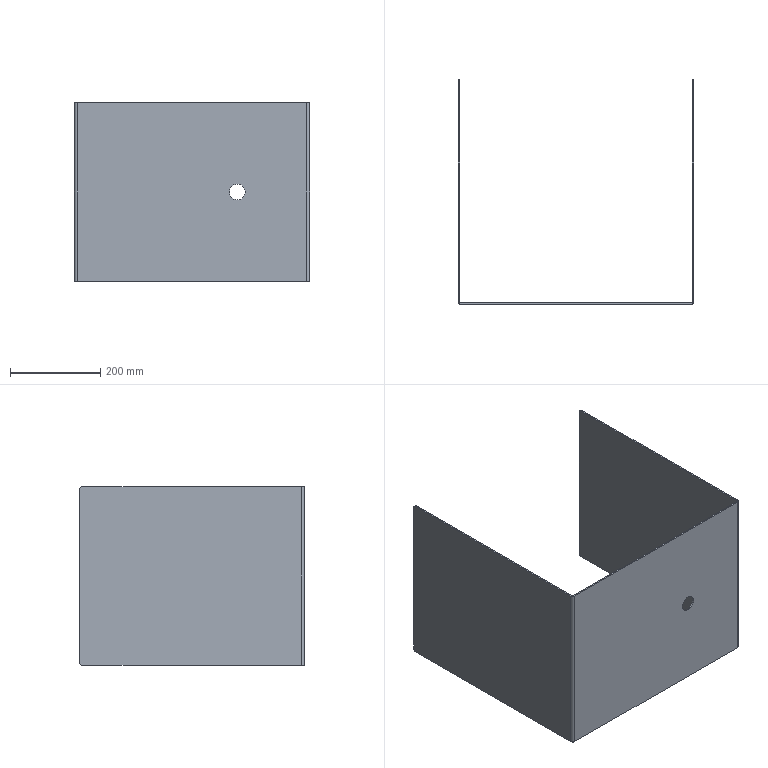Part | SolidWorks | features ICE 2, FlatPattern 1, SMBaseFlange 1, SheetMetal 1 | 1 solid | 28 faces | box 520 x 497 x 394 mm | volume 1774939 mm3 | plane 18 | cylinder 10 | commonest cylinder face diameters 10 x4 6 x2 12 x2 35 x2
STEP:
#1=CARTESIAN_POINT('',(360.,3.,179.5));
#2=VERTEX_POINT('',#1);
#3=CARTESIAN_POINT('',(360.,3.,214.5));
#4=VERTEX_POINT('',#3);
#5=CARTESIAN_POINT('',(360.,3.,197.));
#6=DIRECTION('',(0.,1.,0.));
#7=DIRECTION('',(0.,0.,1.));
#8=AXIS2_PLACEMENT_3D('',#5,#6,#7);
#9=CIRCLE('',#8,17.5);
#10=EDGE_CURVE('',#2,#4,#9,.T.);
#11=ORIENTED_EDGE('',*,*,#10,.T.);
#12=CARTESIAN_POINT('',(360.,0.,214.5));
#13=VERTEX_POINT('',#12);
#14=CARTESIAN_POINT('',(360.,10.,214.5));
#15=DIRECTION('',(0.,-1.,0.));
#16=VECTOR('',#15,1000.);
#17=LINE('',#14,#16);
#18=EDGE_CURVE('',#4,#13,#17,.T.);
#19=ORIENTED_EDGE('',*,*,#18,.T.);
#20=CARTESIAN_POINT('',(360.,0.,179.5));
#21=VERTEX_POINT('',#20);
#22=CARTESIAN_POINT('',(360.,0.,197.));
#23=DIRECTION('',(0.,-1.,0.));
#24=DIRECTION('',(0.,0.,-1.));
#25=AXIS2_PLACEMENT_3D('',#22,#23,#24);
#26=CIRCLE('',#25,17.5);
#27=EDGE_CURVE('',#13,#21,#26,.T.);
#28=ORIENTED_EDGE('',*,*,#27,.T.);
#29=CARTESIAN_POINT('',(360.,10.,179.5));
#30=DIRECTION('',(0.,-1.,0.));
#31=VECTOR('',#30,1000.);
#32=LINE('',#29,#31);
#33=EDGE_CURVE('',#2,#21,#32,.T.);
#34=ORIENTED_EDGE('',*,*,#33,.F.);
#35=EDGE_LOOP('',(#11,#19,#28,#34));
#36=FACE_OUTER_BOUND('',#35,.T.);
#37=CARTESIAN_POINT('',(360.,10.,197.));
#38=DIRECTION('',(0.,-1.,0.));
#39=DIRECTION('',(0.,0.,-1.));
#40=AXIS2_PLACEMENT_3D('',#37,#38,#39);
#41=CYLINDRICAL_SURFACE('',#40,17.5);
#42=ADVANCED_FACE('',(#36),#41,.F.);
#43=CARTESIAN_POINT('',(520.,492.,0.));
#44=VERTEX_POINT('',#43);
#45=CARTESIAN_POINT('',(520.,497.,5.));
#46=VERTEX_POINT('',#45);
#47=CARTESIAN_POINT('',(520.,492.,5.));
#48=DIRECTION('',(1.,0.,0.));
#49=DIRECTION('',(0.,0.,1.));
#50=AXIS2_PLACEMENT_3D('',#47,#48,#49);
#51=CIRCLE('',#50,5.);
#52=EDGE_CURVE('',#44,#46,#51,.T.);
#53=ORIENTED_EDGE('',*,*,#52,.T.);
#54=CARTESIAN_POINT('',(520.,497.,389.));
#55=VERTEX_POINT('',#54);
#56=CARTESIAN_POINT('',(520.,497.,394.));
#57=DIRECTION('',(0.,0.,-1.));
#58=VECTOR('',#57,1000.);
#59=LINE('',#56,#58);
#60=EDGE_CURVE('',#55,#46,#59,.T.);
#61=ORIENTED_EDGE('',*,*,#60,.F.);
#62=CARTESIAN_POINT('',(520.,492.,394.));
#63=VERTEX_POINT('',#62);
#64=CARTESIAN_POINT('',(520.,492.,389.));
#65=DIRECTION('',(1.,0.,0.));
#66=DIRECTION('',(0.,0.,1.));
#67=AXIS2_PLACEMENT_3D('',#64,#65,#66);
#68=CIRCLE('',#67,5.);
#69=EDGE_CURVE('',#55,#63,#68,.T.);
#70=ORIENTED_EDGE('',*,*,#69,.T.);
#71=CARTESIAN_POINT('',(520.,6.,394.));
#72=VERTEX_POINT('',#71);
#73=CARTESIAN_POINT('',(520.,0.,394.));
#74=DIRECTION('',(0.,1.,0.));
#75=VECTOR('',#74,1000.);
#76=LINE('',#73,#75);
#77=EDGE_CURVE('',#72,#63,#76,.T.);
#78=ORIENTED_EDGE('',*,*,#77,.F.);
#79=CARTESIAN_POINT('',(520.,6.,0.));
#80=VERTEX_POINT('',#79);
#81=CARTESIAN_POINT('',(520.,6.,394.));
#82=DIRECTION('',(0.,0.,-1.));
#83=VECTOR('',#82,1000.);
#84=LINE('',#81,#83);
#85=EDGE_CURVE('',#72,#80,#84,.T.);
#86=ORIENTED_EDGE('',*,*,#85,.T.);
#87=CARTESIAN_POINT('',(520.,0.,0.));
#88=DIRECTION('',(0.,1.,0.));
#89=VECTOR('',#88,1000.);
#90=LINE('',#87,#89);
#91=EDGE_CURVE('',#80,#44,#90,.T.);
#92=ORIENTED_EDGE('',*,*,#91,.T.);
#93=EDGE_LOOP('',(#53,#61,#70,#78,#86,#92));
#94=FACE_OUTER_BOUND('',#93,.T.);
#95=CARTESIAN_POINT('',(520.,0.,394.));
#96=DIRECTION('',(-1.,0.,0.));
#97=DIRECTION('',(0.,0.,1.));
#98=AXIS2_PLACEMENT_3D('',#95,#96,#97);
#99=PLANE('',#98);
#100=ADVANCED_FACE('',(#94),#99,.F.);
#101=CARTESIAN_POINT('',(517.,497.,389.));
#102=VERTEX_POINT('',#101);
#103=CARTESIAN_POINT('',(517.,497.,5.));
#104=VERTEX_POINT('',#103);
#105=CARTESIAN_POINT('',(517.,497.,394.));
#106=DIRECTION('',(0.,0.,-1.));
#107=VECTOR('',#106,1000.);
#108=LINE('',#105,#107);
#109=EDGE_CURVE('',#102,#104,#108,.T.);
#110=ORIENTED_EDGE('',*,*,#109,.T.);
#111=CARTESIAN_POINT('',(517.,492.,0.));
#112=VERTEX_POINT('',#111);
#113=CARTESIAN_POINT('',(517.,492.,5.));
#114=DIRECTION('',(1.,0.,0.));
#115=DIRECTION('',(0.,0.,1.));
#116=AXIS2_PLACEMENT_3D('',#113,#114,#115);
#117=CIRCLE('',#116,5.);
#118=EDGE_CURVE('',#112,#104,#117,.T.);
#119=ORIENTED_EDGE('',*,*,#118,.F.);
#120=CARTESIAN_POINT('',(517.,6.,0.));
#121=VERTEX_POINT('',#120);
#122=CARTESIAN_POINT('',(517.,0.,0.));
#123=DIRECTION('',(0.,1.,0.));
#124=VECTOR('',#123,1000.);
#125=LINE('',#122,#124);
#126=EDGE_CURVE('',#121,#112,#125,.T.);
#127=ORIENTED_EDGE('',*,*,#126,.F.);
#128=CARTESIAN_POINT('',(517.,6.,394.));
#129=VERTEX_POINT('',#128);
#130=CARTESIAN_POINT('',(517.,6.,394.));
#131=DIRECTION('',(0.,0.,-1.));
#132=VECTOR('',#131,1000.);
#133=LINE('',#130,#132);
#134=EDGE_CURVE('',#129,#121,#133,.T.);
#135=ORIENTED_EDGE('',*,*,#134,.F.);
#136=CARTESIAN_POINT('',(517.,492.,394.));
#137=VERTEX_POINT('',#136);
#138=CARTESIAN_POINT('',(517.,0.,394.));
#139=DIRECTION('',(0.,1.,0.));
#140=VECTOR('',#139,1000.);
#141=LINE('',#138,#140);
#142=EDGE_CURVE('',#129,#137,#141,.T.);
#143=ORIENTED_EDGE('',*,*,#142,.T.);
#144=CARTESIAN_POINT('',(517.,492.,389.));
#145=DIRECTION('',(1.,0.,0.));
#146=DIRECTION('',(0.,0.,1.));
#147=AXIS2_PLACEMENT_3D('',#144,#145,#146);
#148=CIRCLE('',#147,5.);
#149=EDGE_CURVE('',#102,#137,#148,.T.);
#150=ORIENTED_EDGE('',*,*,#149,.F.);
#151=EDGE_LOOP('',(#110,#119,#127,#135,#143,#150));
#152=FACE_OUTER_BOUND('',#151,.T.);
#153=CARTESIAN_POINT('',(517.,0.,394.));
#154=DIRECTION('',(-1.,0.,0.));
#155=DIRECTION('',(0.,0.,1.));
#156=AXIS2_PLACEMENT_3D('',#153,#154,#155);
#157=PLANE('',#156);
#158=ADVANCED_FACE('',(#152),#157,.T.);
#159=ORIENTED_EDGE('',*,*,#60,.T.);
#160=CARTESIAN_POINT('',(517.,497.,5.));
#161=DIRECTION('',(1.,0.,0.));
#162=VECTOR('',#161,1000.);
#163=LINE('',#160,#162);
#164=EDGE_CURVE('',#104,#46,#163,.T.);
#165=ORIENTED_EDGE('',*,*,#164,.F.);
#166=ORIENTED_EDGE('',*,*,#109,.F.);
#167=CARTESIAN_POINT('',(517.,497.,389.));
#168=DIRECTION('',(1.,0.,0.));
#169=VECTOR('',#168,1000.);
#170=LINE('',#167,#169);
#171=EDGE_CURVE('',#102,#55,#170,.T.);
#172=ORIENTED_EDGE('',*,*,#171,.T.);
#173=EDGE_LOOP('',(#159,#165,#166,#172));
#174=FACE_OUTER_BOUND('',#173,.T.);
#175=CARTESIAN_POINT('',(517.,497.,394.));
#176=DIRECTION('',(0.,1.,0.));
#177=DIRECTION('',(0.,0.,1.));
#178=AXIS2_PLACEMENT_3D('',#175,#176,#177);
#179=PLANE('',#178);
#180=ADVANCED_FACE('',(#174),#179,.T.);
#181=CARTESIAN_POINT('',(3.,492.,0.));
#182=VERTEX_POINT('',#181);
#183=CARTESIAN_POINT('',(3.,6.,0.));
#184=VERTEX_POINT('',#183);
#185=CARTESIAN_POINT('',(3.,0.,0.));
#186=DIRECTION('',(0.,-1.,0.));
#187=VECTOR('',#186,1000.);
#188=LINE('',#185,#187);
#189=EDGE_CURVE('',#182,#184,#188,.T.);
#190=ORIENTED_EDGE('',*,*,#189,.F.);
#191=CARTESIAN_POINT('',(3.,497.,5.));
#192=VERTEX_POINT('',#191);
#193=CARTESIAN_POINT('',(3.,492.,5.));
#194=DIRECTION('',(-1.,0.,0.));
#195=DIRECTION('',(0.,0.,-1.));
#196=AXIS2_PLACEMENT_3D('',#193,#194,#195);
#197=CIRCLE('',#196,5.);
#198=EDGE_CURVE('',#192,#182,#197,.T.);
#199=ORIENTED_EDGE('',*,*,#198,.F.);
#200=CARTESIAN_POINT('',(3.,497.,389.));
#201=VERTEX_POINT('',#200);
#202=CARTESIAN_POINT('',(3.,497.,394.));
#203=DIRECTION('',(0.,0.,-1.));
#204=VECTOR('',#203,1000.);
#205=LINE('',#202,#204);
#206=EDGE_CURVE('',#201,#192,#205,.T.);
#207=ORIENTED_EDGE('',*,*,#206,.F.);
#208=CARTESIAN_POINT('',(3.,492.,394.));
#209=VERTEX_POINT('',#208);
#210=CARTESIAN_POINT('',(3.,492.,389.));
#211=DIRECTION('',(-1.,0.,0.));
#212=DIRECTION('',(0.,0.,-1.));
#213=AXIS2_PLACEMENT_3D('',#210,#211,#212);
#214=CIRCLE('',#213,5.);
#215=EDGE_CURVE('',#209,#201,#214,.T.);
#216=ORIENTED_EDGE('',*,*,#215,.F.);
#217=CARTESIAN_POINT('',(3.,6.,394.));
#218=VERTEX_POINT('',#217);
#219=CARTESIAN_POINT('',(3.,0.,394.));
#220=DIRECTION('',(0.,-1.,0.));
#221=VECTOR('',#220,1000.);
#222=LINE('',#219,#221);
#223=EDGE_CURVE('',#209,#218,#222,.T.);
#224=ORIENTED_EDGE('',*,*,#223,.T.);
#225=CARTESIAN_POINT('',(3.,6.,394.));
#226=DIRECTION('',(0.,0.,-1.));
#227=VECTOR('',#226,1000.);
#228=LINE('',#225,#227);
#229=EDGE_CURVE('',#218,#184,#228,.T.);
#230=ORIENTED_EDGE('',*,*,#229,.T.);
#231=EDGE_LOOP('',(#190,#199,#207,#216,#224,#230));
#232=FACE_OUTER_BOUND('',#231,.T.);
#233=CARTESIAN_POINT('',(3.,0.,394.));
#234=DIRECTION('',(1.,0.,0.));
#235=DIRECTION('',(0.,0.,-1.));
#236=AXIS2_PLACEMENT_3D('',#233,#234,#235);
#237=PLANE('',#236);
#238=ADVANCED_FACE('',(#232),#237,.T.);
#239=CARTESIAN_POINT('',(0.,497.,5.));
#240=VERTEX_POINT('',#239);
#241=CARTESIAN_POINT('',(0.,492.,0.));
#242=VERTEX_POINT('',#241);
#243=CARTESIAN_POINT('',(0.,492.,5.));
#244=DIRECTION('',(-1.,0.,0.));
#245=DIRECTION('',(0.,0.,-1.));
#246=AXIS2_PLACEMENT_3D('',#243,#244,#245);
#247=CIRCLE('',#246,5.);
#248=EDGE_CURVE('',#240,#242,#247,.T.);
#249=ORIENTED_EDGE('',*,*,#248,.T.);
#250=CARTESIAN_POINT('',(0.,6.,0.));
#251=VERTEX_POINT('',#250);
#252=CARTESIAN_POINT('',(0.,0.,0.));
#253=DIRECTION('',(0.,-1.,0.));
#254=VECTOR('',#253,1000.);
#255=LINE('',#252,#254);
#256=EDGE_CURVE('',#242,#251,#255,.T.);
#257=ORIENTED_EDGE('',*,*,#256,.T.);
#258=CARTESIAN_POINT('',(0.,6.,394.));
#259=VERTEX_POINT('',#258);
#260=CARTESIAN_POINT('',(0.,6.,394.));
#261=DIRECTION('',(0.,0.,-1.));
#262=VECTOR('',#261,1000.);
#263=LINE('',#260,#262);
#264=EDGE_CURVE('',#259,#251,#263,.T.);
#265=ORIENTED_EDGE('',*,*,#264,.F.);
#266=CARTESIAN_POINT('',(0.,492.,394.));
#267=VERTEX_POINT('',#266);
#268=CARTESIAN_POINT('',(0.,0.,394.));
#269=DIRECTION('',(0.,-1.,0.));
#270=VECTOR('',#269,1000.);
#271=LINE('',#268,#270);
#272=EDGE_CURVE('',#267,#259,#271,.T.);
#273=ORIENTED_EDGE('',*,*,#272,.F.);
#274=CARTESIAN_POINT('',(0.,497.,389.));
#275=VERTEX_POINT('',#274);
#276=CARTESIAN_POINT('',(0.,492.,389.));
#277=DIRECTION('',(-1.,0.,0.));
#278=DIRECTION('',(0.,0.,-1.));
#279=AXIS2_PLACEMENT_3D('',#276,#277,#278);
#280=CIRCLE('',#279,5.);
#281=EDGE_CURVE('',#267,#275,#280,.T.);
#282=ORIENTED_EDGE('',*,*,#281,.T.);
#283=CARTESIAN_POINT('',(0.,497.,394.));
#284=DIRECTION('',(0.,0.,-1.));
#285=VECTOR('',#284,1000.);
#286=LINE('',#283,#285);
#287=EDGE_CURVE('',#275,#240,#286,.T.);
#288=ORIENTED_EDGE('',*,*,#287,.T.);
#289=EDGE_LOOP('',(#249,#257,#265,#273,#282,#288));
#290=FACE_OUTER_BOUND('',#289,.T.);
#291=CARTESIAN_POINT('',(0.,0.,394.));
#292=DIRECTION('',(1.,0.,0.));
#293=DIRECTION('',(0.,0.,-1.));
#294=AXIS2_PLACEMENT_3D('',#291,#292,#293);
#295=PLANE('',#294);
#296=ADVANCED_FACE('',(#290),#295,.F.);
#297=ORIENTED_EDGE('',*,*,#77,.T.);
#298=CARTESIAN_POINT('',(517.,492.,394.));
#299=DIRECTION('',(1.,0.,0.));
#300=VECTOR('',#299,1000.);
#301=LINE('',#298,#300);
#302=EDGE_CURVE('',#137,#63,#301,.T.);
#303=ORIENTED_EDGE('',*,*,#302,.F.);
#304=ORIENTED_EDGE('',*,*,#142,.F.);
#305=CARTESIAN_POINT('',(517.,6.,394.));
#306=DIRECTION('',(1.,0.,0.));
#307=VECTOR('',#306,1000.);
#308=LINE('',#305,#307);
#309=EDGE_CURVE('',#129,#72,#308,.T.);
#310=ORIENTED_EDGE('',*,*,#309,.T.);
#311=EDGE_LOOP('',(#297,#303,#304,#310));
#312=FACE_OUTER_BOUND('',#311,.T.);
#313=CARTESIAN_POINT('',(514.,6.,394.));
#314=DIRECTION('',(0.,0.,1.));
#315=DIRECTION('',(1.,0.,0.));
#316=AXIS2_PLACEMENT_3D('',#313,#314,#315);
#317=PLANE('',#316);
#318=ADVANCED_FACE('',(#312),#317,.T.);
#319=CARTESIAN_POINT('',(3.,497.,5.));
#320=DIRECTION('',(-1.,0.,0.));
#321=VECTOR('',#320,1000.);
#322=LINE('',#319,#321);
#323=EDGE_CURVE('',#192,#240,#322,.T.);
#324=ORIENTED_EDGE('',*,*,#323,.T.);
#325=ORIENTED_EDGE('',*,*,#287,.F.);
#326=CARTESIAN_POINT('',(3.,497.,389.));
#327=DIRECTION('',(-1.,0.,0.));
#328=VECTOR('',#327,1000.);
#329=LINE('',#326,#328);
#330=EDGE_CURVE('',#201,#275,#329,.T.);
#331=ORIENTED_EDGE('',*,*,#330,.F.);
#332=ORIENTED_EDGE('',*,*,#206,.T.);
#333=EDGE_LOOP('',(#324,#325,#331,#332));
#334=FACE_OUTER_BOUND('',#333,.T.);
#335=CARTESIAN_POINT('',(0.,497.,394.));
#336=DIRECTION('',(0.,1.,0.));
#337=DIRECTION('',(0.,0.,1.));
#338=AXIS2_PLACEMENT_3D('',#335,#336,#337);
#339=PLANE('',#338);
#340=ADVANCED_FACE('',(#334),#339,.T.);
#341=CARTESIAN_POINT('',(0.,6.,394.));
#342=DIRECTION('',(1.,0.,0.));
#343=VECTOR('',#342,1000.);
#344=LINE('',#341,#343);
#345=EDGE_CURVE('',#259,#218,#344,.T.);
#346=ORIENTED_EDGE('',*,*,#345,.F.);
#347=CARTESIAN_POINT('',(6.,0.,394.));
#348=VERTEX_POINT('',#347);
#349=CARTESIAN_POINT('',(6.,6.,394.));
#350=DIRECTION('',(0.,0.,1.));
#351=DIRECTION('',(-1.,0.,0.));
#352=AXIS2_PLACEMENT_3D('',#349,#350,#351);
#353=CIRCLE('',#352,6.);
#354=EDGE_CURVE('',#259,#348,#353,.T.);
#355=ORIENTED_EDGE('',*,*,#354,.T.);
#356=CARTESIAN_POINT('',(6.,3.,394.));
#357=VERTEX_POINT('',#356);
#358=CARTESIAN_POINT('',(6.,3.,394.));
#359=DIRECTION('',(0.,-1.,0.));
#360=VECTOR('',#359,1000.);
#361=LINE('',#358,#360);
#362=EDGE_CURVE('',#357,#348,#361,.T.);
#363=ORIENTED_EDGE('',*,*,#362,.F.);
#364=CARTESIAN_POINT('',(6.,6.,394.));
#365=DIRECTION('',(0.,0.,1.));
#366=DIRECTION('',(1.,0.,0.));
#367=AXIS2_PLACEMENT_3D('',#364,#365,#366);
#368=CIRCLE('',#367,3.);
#369=EDGE_CURVE('',#218,#357,#368,.T.);
#370=ORIENTED_EDGE('',*,*,#369,.F.);
#371=EDGE_LOOP('',(#346,#355,#363,#370));
#372=FACE_OUTER_BOUND('',#371,.T.);
#373=CARTESIAN_POINT('',(0.,6.,394.));
#374=DIRECTION('',(0.,0.,1.));
#375=DIRECTION('',(1.,0.,0.));
#376=AXIS2_PLACEMENT_3D('',#373,#374,#375);
#377=PLANE('',#376);
#378=ADVANCED_FACE('',(#372),#377,.T.);
#379=CARTESIAN_POINT('',(3.,492.,394.));
#380=DIRECTION('',(-1.,0.,0.));
#381=VECTOR('',#380,1000.);
#382=LINE('',#379,#381);
#383=EDGE_CURVE('',#209,#267,#382,.T.);
#384=ORIENTED_EDGE('',*,*,#383,.T.);
#385=ORIENTED_EDGE('',*,*,#272,.T.);
#386=ORIENTED_EDGE('',*,*,#345,.T.);
#387=ORIENTED_EDGE('',*,*,#223,.F.);
#388=EDGE_LOOP('',(#384,#385,#386,#387));
#389=FACE_OUTER_BOUND('',#388,.T.);
#390=CARTESIAN_POINT('',(6.,3.,394.));
#391=DIRECTION('',(0.,0.,1.));
#392=DIRECTION('',(1.,0.,0.));
#393=AXIS2_PLACEMENT_3D('',#390,#391,#392);
#394=PLANE('',#393);
#395=ADVANCED_FACE('',(#389),#394,.T.);
#396=CARTESIAN_POINT('',(6.,0.,0.));
#397=VERTEX_POINT('',#396);
#398=CARTESIAN_POINT('',(6.,3.,0.));
#399=VERTEX_POINT('',#398);
#400=CARTESIAN_POINT('',(6.,0.,0.));
#401=DIRECTION('',(0.,1.,0.));
#402=VECTOR('',#401,1000.);
#403=LINE('',#400,#402);
#404=EDGE_CURVE('',#397,#399,#403,.T.);
#405=ORIENTED_EDGE('',*,*,#404,.F.);
#406=CARTESIAN_POINT('',(6.,6.,0.));
#407=DIRECTION('',(0.,0.,1.));
#408=DIRECTION('',(-1.,0.,0.));
#409=AXIS2_PLACEMENT_3D('',#406,#407,#408);
#410=CIRCLE('',#409,6.);
#411=EDGE_CURVE('',#251,#397,#410,.T.);
#412=ORIENTED_EDGE('',*,*,#411,.F.);
#413=CARTESIAN_POINT('',(3.,6.,0.));
#414=DIRECTION('',(-1.,0.,0.));
#415=VECTOR('',#414,1000.);
#416=LINE('',#413,#415);
#417=EDGE_CURVE('',#184,#251,#416,.T.);
#418=ORIENTED_EDGE('',*,*,#417,.F.);
#419=CARTESIAN_POINT('',(6.,6.,0.));
#420=DIRECTION('',(0.,0.,1.));
#421=DIRECTION('',(1.,0.,0.));
#422=AXIS2_PLACEMENT_3D('',#419,#420,#421);
#423=CIRCLE('',#422,3.);
#424=EDGE_CURVE('',#184,#399,#423,.T.);
#425=ORIENTED_EDGE('',*,*,#424,.T.);
#426=EDGE_LOOP('',(#405,#412,#418,#425));
#427=FACE_OUTER_BOUND('',#426,.T.);
#428=CARTESIAN_POINT('',(6.,0.,0.));
#429=DIRECTION('',(0.,0.,-1.));
#430=DIRECTION('',(-1.,0.,0.));
#431=AXIS2_PLACEMENT_3D('',#428,#429,#430);
#432=PLANE('',#431);
#433=ADVANCED_FACE('',(#427),#432,.T.);
#434=CARTESIAN_POINT('',(514.,0.,0.));
#435=VERTEX_POINT('',#434);
#436=CARTESIAN_POINT('',(0.,0.,0.));
#437=DIRECTION('',(1.,0.,0.));
#438=VECTOR('',#437,1000.);
#439=LINE('',#436,#438);
#440=EDGE_CURVE('',#397,#435,#439,.T.);
#441=ORIENTED_EDGE('',*,*,#440,.F.);
#442=ORIENTED_EDGE('',*,*,#404,.T.);
#443=CARTESIAN_POINT('',(514.,3.,0.));
#444=VERTEX_POINT('',#443);
#445=CARTESIAN_POINT('',(0.,3.,0.));
#446=DIRECTION('',(1.,0.,0.));
#447=VECTOR('',#446,1000.);
#448=LINE('',#445,#447);
#449=EDGE_CURVE('',#399,#444,#448,.T.);
#450=ORIENTED_EDGE('',*,*,#449,.T.);
#451=CARTESIAN_POINT('',(514.,3.,0.));
#452=DIRECTION('',(0.,-1.,0.));
#453=VECTOR('',#452,1000.);
#454=LINE('',#451,#453);
#455=EDGE_CURVE('',#444,#435,#454,.T.);
#456=ORIENTED_EDGE('',*,*,#455,.T.);
#457=EDGE_LOOP('',(#441,#442,#450,#456));
#458=FACE_OUTER_BOUND('',#457,.T.);
#459=CARTESIAN_POINT('',(3.,6.,0.));
#460=DIRECTION('',(0.,0.,-1.));
#461=DIRECTION('',(-1.,0.,0.));
#462=AXIS2_PLACEMENT_3D('',#459,#460,#461);
#463=PLANE('',#462);
#464=ADVANCED_FACE('',(#458),#463,.T.);
#465=CARTESIAN_POINT('',(514.,0.,394.));
#466=VERTEX_POINT('',#465);
#467=CARTESIAN_POINT('',(514.,3.,394.));
#468=VERTEX_POINT('',#467);
#469=CARTESIAN_POINT('',(514.,0.,394.));
#470=DIRECTION('',(0.,1.,0.));
#471=VECTOR('',#470,1000.);
#472=LINE('',#469,#471);
#473=EDGE_CURVE('',#466,#468,#472,.T.);
#474=ORIENTED_EDGE('',*,*,#473,.F.);
#475=CARTESIAN_POINT('',(514.,6.,394.));
#476=DIRECTION('',(0.,0.,1.));
#477=DIRECTION('',(-1.,0.,0.));
#478=AXIS2_PLACEMENT_3D('',#475,#476,#477);
#479=CIRCLE('',#478,6.);
#480=EDGE_CURVE('',#466,#72,#479,.T.);
#481=ORIENTED_EDGE('',*,*,#480,.T.);
#482=ORIENTED_EDGE('',*,*,#309,.F.);
#483=CARTESIAN_POINT('',(514.,6.,394.));
#484=DIRECTION('',(0.,0.,1.));
#485=DIRECTION('',(1.,0.,0.));
#486=AXIS2_PLACEMENT_3D('',#483,#484,#485);
#487=CIRCLE('',#486,3.);
#488=EDGE_CURVE('',#468,#129,#487,.T.);
#489=ORIENTED_EDGE('',*,*,#488,.F.);
#490=EDGE_LOOP('',(#474,#481,#482,#489));
#491=FACE_OUTER_BOUND('',#490,.T.);
#492=CARTESIAN_POINT('',(514.,0.,394.));
#493=DIRECTION('',(0.,0.,1.));
#494=DIRECTION('',(1.,0.,0.));
#495=AXIS2_PLACEMENT_3D('',#492,#493,#494);
#496=PLANE('',#495);
#497=ADVANCED_FACE('',(#491),#496,.T.);
#498=CARTESIAN_POINT('',(0.,0.,394.));
#499=DIRECTION('',(1.,0.,0.));
#500=VECTOR('',#499,1000.);
#501=LINE('',#498,#500);
#502=EDGE_CURVE('',#348,#466,#501,.T.);
#503=ORIENTED_EDGE('',*,*,#502,.T.);
#504=ORIENTED_EDGE('',*,*,#473,.T.);
#505=CARTESIAN_POINT('',(0.,3.,394.));
#506=DIRECTION('',(1.,0.,0.));
#507=VECTOR('',#506,1000.);
#508=LINE('',#505,#507);
#509=EDGE_CURVE('',#357,#468,#508,.T.);
#510=ORIENTED_EDGE('',*,*,#509,.F.);
#511=ORIENTED_EDGE('',*,*,#362,.T.);
#512=EDGE_LOOP('',(#503,#504,#510,#511));
#513=FACE_OUTER_BOUND('',#512,.T.);
#514=CARTESIAN_POINT('',(517.,6.,394.));
#515=DIRECTION('',(0.,0.,1.));
#516=DIRECTION('',(1.,0.,0.));
#517=AXIS2_PLACEMENT_3D('',#514,#515,#516);
#518=PLANE('',#517);
#519=ADVANCED_FACE('',(#513),#518,.T.);
#520=CARTESIAN_POINT('',(520.,6.,0.));
#521=DIRECTION('',(-1.,0.,0.));
#522=VECTOR('',#521,1000.);
#523=LINE('',#520,#522);
#524=EDGE_CURVE('',#80,#121,#523,.T.);
#525=ORIENTED_EDGE('',*,*,#524,.F.);
#526=CARTESIAN_POINT('',(514.,6.,0.));
#527=DIRECTION('',(0.,0.,1.));
#528=DIRECTION('',(-1.,0.,0.));
#529=AXIS2_PLACEMENT_3D('',#526,#527,#528);
#530=CIRCLE('',#529,6.);
#531=EDGE_CURVE('',#435,#80,#530,.T.);
#532=ORIENTED_EDGE('',*,*,#531,.F.);
#533=ORIENTED_EDGE('',*,*,#455,.F.);
#534=CARTESIAN_POINT('',(514.,6.,0.));
#535=DIRECTION('',(0.,0.,1.));
#536=DIRECTION('',(1.,0.,0.));
#537=AXIS2_PLACEMENT_3D('',#534,#535,#536);
#538=CIRCLE('',#537,3.);
#539=EDGE_CURVE('',#444,#121,#538,.T.);
#540=ORIENTED_EDGE('',*,*,#539,.T.);
#541=EDGE_LOOP('',(#525,#532,#533,#540));
#542=FACE_OUTER_BOUND('',#541,.T.);
#543=CARTESIAN_POINT('',(520.,6.,0.));
#544=DIRECTION('',(0.,0.,-1.));
#545=DIRECTION('',(-1.,0.,0.));
#546=AXIS2_PLACEMENT_3D('',#543,#544,#545);
#547=PLANE('',#546);
#548=ADVANCED_FACE('',(#542),#547,.T.);
#549=CARTESIAN_POINT('',(517.,492.,0.));
#550=DIRECTION('',(1.,0.,0.));
#551=VECTOR('',#550,1000.);
#552=LINE('',#549,#551);
#553=EDGE_CURVE('',#112,#44,#552,.T.);
#554=ORIENTED_EDGE('',*,*,#553,.T.);
#555=ORIENTED_EDGE('',*,*,#91,.F.);
#556=ORIENTED_EDGE('',*,*,#524,.T.);
#557=ORIENTED_EDGE('',*,*,#126,.T.);
#558=EDGE_LOOP('',(#554,#555,#556,#557));
#559=FACE_OUTER_BOUND('',#558,.T.);
#560=CARTESIAN_POINT('',(514.,3.,0.));
#561=DIRECTION('',(0.,0.,-1.));
#562=DIRECTION('',(-1.,0.,0.));
#563=AXIS2_PLACEMENT_3D('',#560,#561,#562);
#564=PLANE('',#563);
#565=ADVANCED_FACE('',(#559),#564,.T.);
#566=ORIENTED_EDGE('',*,*,#539,.F.);
#567=CARTESIAN_POINT('',(514.,3.,394.));
#568=DIRECTION('',(0.,0.,-1.));
#569=VECTOR('',#568,1000.);
#570=LINE('',#567,#569);
#571=EDGE_CURVE('',#468,#444,#570,.T.);
#572=ORIENTED_EDGE('',*,*,#571,.F.);
#573=ORIENTED_EDGE('',*,*,#488,.T.);
#574=ORIENTED_EDGE('',*,*,#134,.T.);
#575=EDGE_LOOP('',(#566,#572,#573,#574));
#576=FACE_OUTER_BOUND('',#575,.T.);
#577=CARTESIAN_POINT('',(514.,6.,394.));
#578=DIRECTION('',(0.,0.,-1.));
#579=DIRECTION('',(-1.,0.,0.));
#580=AXIS2_PLACEMENT_3D('',#577,#578,#579);
#581=CYLINDRICAL_SURFACE('',#580,3.);
#582=ADVANCED_FACE('',(#576),#581,.F.);
#583=ORIENTED_EDGE('',*,*,#10,.F.);
#584=CARTESIAN_POINT('',(360.,3.,197.));
#585=DIRECTION('',(0.,1.,0.));
#586=DIRECTION('',(0.,0.,1.));
#587=AXIS2_PLACEMENT_3D('',#584,#585,#586);
#588=CIRCLE('',#587,17.5);
#589=EDGE_CURVE('',#4,#2,#588,.T.);
#590=ORIENTED_EDGE('',*,*,#589,.F.);
#591=EDGE_LOOP('',(#583,#590));
#592=FACE_BOUND('',#591,.T.);
#593=ORIENTED_EDGE('',*,*,#449,.F.);
#594=CARTESIAN_POINT('',(6.,3.,394.));
#595=DIRECTION('',(0.,0.,-1.));
#596=VECTOR('',#595,1000.);
#597=LINE('',#594,#596);
#598=EDGE_CURVE('',#357,#399,#597,.T.);
#599=ORIENTED_EDGE('',*,*,#598,.F.);
#600=ORIENTED_EDGE('',*,*,#509,.T.);
#601=ORIENTED_EDGE('',*,*,#571,.T.);
#602=EDGE_LOOP('',(#593,#599,#600,#601));
#603=FACE_OUTER_BOUND('',#602,.T.);
#604=CARTESIAN_POINT('',(0.,3.,394.));
#605=DIRECTION('',(0.,1.,0.));
#606=DIRECTION('',(0.,0.,1.));
#607=AXIS2_PLACEMENT_3D('',#604,#605,#606);
#608=PLANE('',#607);
#609=ADVANCED_FACE('',(#592,#603),#608,.T.);
#610=ORIENTED_EDGE('',*,*,#424,.F.);
#611=ORIENTED_EDGE('',*,*,#229,.F.);
#612=ORIENTED_EDGE('',*,*,#369,.T.);
#613=ORIENTED_EDGE('',*,*,#598,.T.);
#614=EDGE_LOOP('',(#610,#611,#612,#613));
#615=FACE_OUTER_BOUND('',#614,.T.);
#616=CARTESIAN_POINT('',(6.,6.,394.));
#617=DIRECTION('',(0.,0.,-1.));
#618=DIRECTION('',(-1.,0.,0.));
#619=AXIS2_PLACEMENT_3D('',#616,#617,#618);
#620=CYLINDRICAL_SURFACE('',#619,3.);
#621=ADVANCED_FACE('',(#615),#620,.F.);
#622=ORIENTED_EDGE('',*,*,#411,.T.);
#623=CARTESIAN_POINT('',(6.,0.,394.));
#624=DIRECTION('',(0.,0.,-1.));
#625=VECTOR('',#624,1000.);
#626=LINE('',#623,#625);
#627=EDGE_CURVE('',#348,#397,#626,.T.);
#628=ORIENTED_EDGE('',*,*,#627,.F.);
#629=ORIENTED_EDGE('',*,*,#354,.F.);
#630=ORIENTED_EDGE('',*,*,#264,.T.);
#631=EDGE_LOOP('',(#622,#628,#629,#630));
#632=FACE_OUTER_BOUND('',#631,.T.);
#633=CARTESIAN_POINT('',(6.,6.,394.));
#634=DIRECTION('',(0.,0.,-1.));
#635=DIRECTION('',(-1.,0.,0.));
#636=AXIS2_PLACEMENT_3D('',#633,#634,#635);
#637=CYLINDRICAL_SURFACE('',#636,6.);
#638=ADVANCED_FACE('',(#632),#637,.T.);
#639=CARTESIAN_POINT('',(360.,0.,197.));
#640=DIRECTION('',(0.,-1.,0.));
#641=DIRECTION('',(0.,0.,-1.));
#642=AXIS2_PLACEMENT_3D('',#639,#640,#641);
#643=CIRCLE('',#642,17.5);
#644=EDGE_CURVE('',#21,#13,#643,.T.);
#645=ORIENTED_EDGE('',*,*,#644,.F.);
#646=ORIENTED_EDGE('',*,*,#27,.F.);
#647=EDGE_LOOP('',(#645,#646));
#648=FACE_BOUND('',#647,.T.);
#649=ORIENTED_EDGE('',*,*,#440,.T.);
#650=CARTESIAN_POINT('',(514.,0.,394.));
#651=DIRECTION('',(0.,0.,-1.));
#652=VECTOR('',#651,1000.);
#653=LINE('',#650,#652);
#654=EDGE_CURVE('',#466,#435,#653,.T.);
#655=ORIENTED_EDGE('',*,*,#654,.F.);
#656=ORIENTED_EDGE('',*,*,#502,.F.);
#657=ORIENTED_EDGE('',*,*,#627,.T.);
#658=EDGE_LOOP('',(#649,#655,#656,#657));
#659=FACE_OUTER_BOUND('',#658,.T.);
#660=CARTESIAN_POINT('',(0.,0.,394.));
#661=DIRECTION('',(0.,1.,0.));
#662=DIRECTION('',(0.,0.,1.));
#663=AXIS2_PLACEMENT_3D('',#660,#661,#662);
#664=PLANE('',#663);
#665=ADVANCED_FACE('',(#648,#659),#664,.F.);
#666=ORIENTED_EDGE('',*,*,#531,.T.);
#667=ORIENTED_EDGE('',*,*,#85,.F.);
#668=ORIENTED_EDGE('',*,*,#480,.F.);
#669=ORIENTED_EDGE('',*,*,#654,.T.);
#670=EDGE_LOOP('',(#666,#667,#668,#669));
#671=FACE_OUTER_BOUND('',#670,.T.);
#672=CARTESIAN_POINT('',(514.,6.,394.));
#673=DIRECTION('',(0.,0.,-1.));
#674=DIRECTION('',(-1.,0.,0.));
#675=AXIS2_PLACEMENT_3D('',#672,#673,#674);
#676=CYLINDRICAL_SURFACE('',#675,6.);
#677=ADVANCED_FACE('',(#671),#676,.T.);
#678=ORIENTED_EDGE('',*,*,#256,.F.);
#679=CARTESIAN_POINT('',(3.,492.,0.));
#680=DIRECTION('',(-1.,0.,0.));
#681=VECTOR('',#680,1000.);
#682=LINE('',#679,#681);
#683=EDGE_CURVE('',#182,#242,#682,.T.);
#684=ORIENTED_EDGE('',*,*,#683,.F.);
#685=ORIENTED_EDGE('',*,*,#189,.T.);
#686=ORIENTED_EDGE('',*,*,#417,.T.);
#687=EDGE_LOOP('',(#678,#684,#685,#686));
#688=FACE_OUTER_BOUND('',#687,.T.);
#689=CARTESIAN_POINT('',(514.,6.,0.));
#690=DIRECTION('',(0.,0.,1.));
#691=DIRECTION('',(1.,0.,0.));
#692=AXIS2_PLACEMENT_3D('',#689,#690,#691);
#693=PLANE('',#692);
#694=ADVANCED_FACE('',(#688),#693,.F.);
#695=ORIENTED_EDGE('',*,*,#18,.F.);
#696=ORIENTED_EDGE('',*,*,#589,.T.);
#697=ORIENTED_EDGE('',*,*,#33,.T.);
#698=ORIENTED_EDGE('',*,*,#644,.T.);
#699=EDGE_LOOP('',(#695,#696,#697,#698));
#700=FACE_OUTER_BOUND('',#699,.T.);
#701=CARTESIAN_POINT('',(360.,10.,197.));
#702=DIRECTION('',(0.,-1.,0.));
#703=DIRECTION('',(0.,0.,-1.));
#704=AXIS2_PLACEMENT_3D('',#701,#702,#703);
#705=CYLINDRICAL_SURFACE('',#704,17.5);
#706=ADVANCED_FACE('',(#700),#705,.F.);
#707=ORIENTED_EDGE('',*,*,#215,.T.);
#708=ORIENTED_EDGE('',*,*,#330,.T.);
#709=ORIENTED_EDGE('',*,*,#281,.F.);
#710=ORIENTED_EDGE('',*,*,#383,.F.);
#711=EDGE_LOOP('',(#707,#708,#709,#710));
#712=FACE_OUTER_BOUND('',#711,.T.);
#713=CARTESIAN_POINT('',(3.,492.,389.));
#714=DIRECTION('',(1.,0.,0.));
#715=DIRECTION('',(0.,0.,-1.));
#716=AXIS2_PLACEMENT_3D('',#713,#714,#715);
#717=CYLINDRICAL_SURFACE('',#716,5.);
#718=ADVANCED_FACE('',(#712),#717,.T.);
#719=ORIENTED_EDGE('',*,*,#149,.T.);
#720=ORIENTED_EDGE('',*,*,#302,.T.);
#721=ORIENTED_EDGE('',*,*,#69,.F.);
#722=ORIENTED_EDGE('',*,*,#171,.F.);
#723=EDGE_LOOP('',(#719,#720,#721,#722));
#724=FACE_OUTER_BOUND('',#723,.T.);
#725=CARTESIAN_POINT('',(517.,492.,389.));
#726=DIRECTION('',(-1.,0.,0.));
#727=DIRECTION('',(0.,0.,1.));
#728=AXIS2_PLACEMENT_3D('',#725,#726,#727);
#729=CYLINDRICAL_SURFACE('',#728,5.);
#730=ADVANCED_FACE('',(#724),#729,.T.);
#731=ORIENTED_EDGE('',*,*,#198,.T.);
#732=ORIENTED_EDGE('',*,*,#683,.T.);
#733=ORIENTED_EDGE('',*,*,#248,.F.);
#734=ORIENTED_EDGE('',*,*,#323,.F.);
#735=EDGE_LOOP('',(#731,#732,#733,#734));
#736=FACE_OUTER_BOUND('',#735,.T.);
#737=CARTESIAN_POINT('',(3.,492.,5.));
#738=DIRECTION('',(1.,0.,0.));
#739=DIRECTION('',(0.,0.,-1.));
#740=AXIS2_PLACEMENT_3D('',#737,#738,#739);
#741=CYLINDRICAL_SURFACE('',#740,5.);
#742=ADVANCED_FACE('',(#736),#741,.T.);
#743=ORIENTED_EDGE('',*,*,#118,.T.);
#744=ORIENTED_EDGE('',*,*,#164,.T.);
#745=ORIENTED_EDGE('',*,*,#52,.F.);
#746=ORIENTED_EDGE('',*,*,#553,.F.);
#747=EDGE_LOOP('',(#743,#744,#745,#746));
#748=FACE_OUTER_BOUND('',#747,.T.);
#749=CARTESIAN_POINT('',(517.,492.,5.));
#750=DIRECTION('',(-1.,0.,0.));
#751=DIRECTION('',(0.,0.,1.));
#752=AXIS2_PLACEMENT_3D('',#749,#750,#751);
#753=CYLINDRICAL_SURFACE('',#752,5.);
#754=ADVANCED_FACE('',(#748),#753,.T.);
#755=CLOSED_SHELL('',(#42,#100,#158,#180,#238,#296,#318,#340,#378,#395,#433,#464,#497,#519,#548,#565,#582,#609,#621,#638,#665,#677,#694,#706,#718,#730,#742,#754));
#756=MANIFOLD_SOLID_BREP('',#755);
#757=CARTESIAN_POINT('',(0.,0.,0.));
#758=DIRECTION('',(0.,0.,1.));
#759=DIRECTION('',(1.,0.,0.));
#760=AXIS2_PLACEMENT_3D('',#757,#758,#759);
#761=(LENGTH_UNIT()NAMED_UNIT(*)SI_UNIT(.MILLI.,.METRE.));
#762=UNCERTAINTY_MEASURE_WITH_UNIT(LENGTH_MEASURE(0.00001),#761,'','');
#763=(NAMED_UNIT(*)PLANE_ANGLE_UNIT()SI_UNIT($,.RADIAN.));
#764=(NAMED_UNIT(*)SI_UNIT($,.STERADIAN.)SOLID_ANGLE_UNIT());
#765=(GEOMETRIC_REPRESENTATION_CONTEXT(3)GLOBAL_UNCERTAINTY_ASSIGNED_CONTEXT((#762))GLOBAL_UNIT_ASSIGNED_CONTEXT((#761,#763,#764))REPRESENTATION_CONTEXT('',''));
#766=ADVANCED_BREP_SHAPE_REPRESENTATION('',(#756,#760),#765);